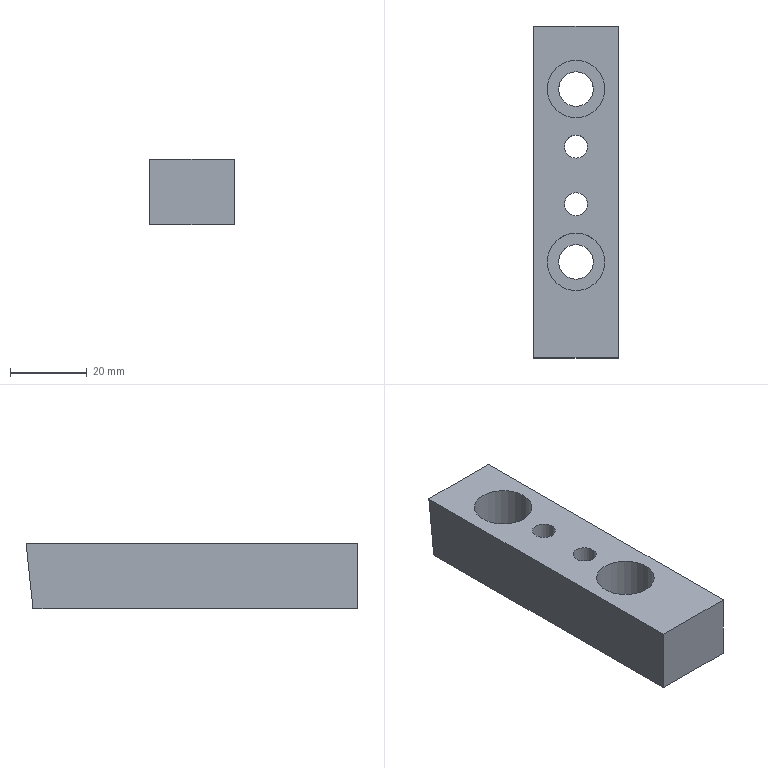Part | NX | features DATUM_CSYS 4, SKETCH 3, CBORE_HOLE 2, HOLE PACKAGE 2, SIMPLE HOLE 2, EXTRUDE 1 | 1 solid | 14 faces | box 22 x 86.4 x 17 mm | volume 26138 mm3 | plane 8 | cylinder 6 | commonest cylinder face diameters 6 x2 9 x2 15 x2
STEP:
#1=CARTESIAN_POINT('',(0.,-43.2,8.5));
#2=VERTEX_POINT('',#1);
#3=CARTESIAN_POINT('',(0.,-43.2,-8.5));
#4=VERTEX_POINT('',#3);
#5=CARTESIAN_POINT('',(0.,-43.2,8.5));
#6=DIRECTION('',(0.,0.,-1.));
#7=VECTOR('',#6,1000.);
#8=LINE('',#5,#7);
#9=EDGE_CURVE('',#2,#4,#8,.T.);
#10=ORIENTED_EDGE('',*,*,#9,.T.);
#11=CARTESIAN_POINT('',(22.,-43.2,-8.5));
#12=VERTEX_POINT('',#11);
#13=CARTESIAN_POINT('',(22.,-43.2,-8.5));
#14=DIRECTION('',(-1.,0.,0.));
#15=VECTOR('',#14,1000.);
#16=LINE('',#13,#15);
#17=EDGE_CURVE('',#12,#4,#16,.T.);
#18=ORIENTED_EDGE('',*,*,#17,.F.);
#19=CARTESIAN_POINT('',(22.,-43.2,8.5));
#20=VERTEX_POINT('',#19);
#21=CARTESIAN_POINT('',(22.,-43.2,8.5));
#22=DIRECTION('',(0.,0.,-1.));
#23=VECTOR('',#22,1000.);
#24=LINE('',#21,#23);
#25=EDGE_CURVE('',#20,#12,#24,.T.);
#26=ORIENTED_EDGE('',*,*,#25,.F.);
#27=CARTESIAN_POINT('',(22.,-43.2,8.5));
#28=DIRECTION('',(-1.,0.,0.));
#29=VECTOR('',#28,1000.);
#30=LINE('',#27,#29);
#31=EDGE_CURVE('',#20,#2,#30,.T.);
#32=ORIENTED_EDGE('',*,*,#31,.T.);
#33=EDGE_LOOP('',(#10,#18,#26,#32));
#34=FACE_BOUND('',#33,.T.);
#35=CARTESIAN_POINT('',(22.,-43.2,8.5));
#36=DIRECTION('',(0.,1.,0.));
#37=DIRECTION('',(0.,0.,1.));
#38=AXIS2_PLACEMENT_3D('',#35,#36,#37);
#39=PLANE('',#38);
#40=ADVANCED_FACE('',(#34),#39,.F.);
#41=CARTESIAN_POINT('',(11.,8.8,-8.5));
#42=VERTEX_POINT('',#41);
#43=CARTESIAN_POINT('',(11.,11.8,-8.5));
#44=DIRECTION('',(0.,0.,1.));
#45=DIRECTION('',(0.,-1.,0.));
#46=AXIS2_PLACEMENT_3D('',#43,#44,#45);
#47=CIRCLE('',#46,3.);
#48=EDGE_CURVE('',#42,#42,#47,.T.);
#49=ORIENTED_EDGE('',*,*,#48,.T.);
#50=EDGE_LOOP('',(#49));
#51=FACE_BOUND('',#50,.T.);
#52=CARTESIAN_POINT('',(11.,-6.2,-8.5));
#53=VERTEX_POINT('',#52);
#54=CARTESIAN_POINT('',(11.,-3.2,-8.5));
#55=DIRECTION('',(0.,0.,1.));
#56=DIRECTION('',(0.,-1.,0.));
#57=AXIS2_PLACEMENT_3D('',#54,#55,#56);
#58=CIRCLE('',#57,3.);
#59=EDGE_CURVE('',#53,#53,#58,.T.);
#60=ORIENTED_EDGE('',*,*,#59,.T.);
#61=EDGE_LOOP('',(#60));
#62=FACE_BOUND('',#61,.T.);
#63=CARTESIAN_POINT('',(11.,22.3,-8.5));
#64=VERTEX_POINT('',#63);
#65=CARTESIAN_POINT('',(11.,26.8,-8.5));
#66=DIRECTION('',(0.,0.,1.));
#67=DIRECTION('',(0.,-1.,0.));
#68=AXIS2_PLACEMENT_3D('',#65,#66,#67);
#69=CIRCLE('',#68,4.5);
#70=EDGE_CURVE('',#64,#64,#69,.T.);
#71=ORIENTED_EDGE('',*,*,#70,.T.);
#72=EDGE_LOOP('',(#71));
#73=FACE_BOUND('',#72,.T.);
#74=CARTESIAN_POINT('',(11.,-22.7,-8.5));
#75=VERTEX_POINT('',#74);
#76=CARTESIAN_POINT('',(11.,-18.2,-8.5));
#77=DIRECTION('',(0.,0.,1.));
#78=DIRECTION('',(0.,-1.,0.));
#79=AXIS2_PLACEMENT_3D('',#76,#77,#78);
#80=CIRCLE('',#79,4.5);
#81=EDGE_CURVE('',#75,#75,#80,.T.);
#82=ORIENTED_EDGE('',*,*,#81,.T.);
#83=EDGE_LOOP('',(#82));
#84=FACE_BOUND('',#83,.T.);
#85=CARTESIAN_POINT('',(0.,41.4,-8.5));
#86=VERTEX_POINT('',#85);
#87=CARTESIAN_POINT('',(0.,-43.2,-8.5));
#88=DIRECTION('',(0.,1.,0.));
#89=VECTOR('',#88,1000.);
#90=LINE('',#87,#89);
#91=EDGE_CURVE('',#4,#86,#90,.T.);
#92=ORIENTED_EDGE('',*,*,#91,.T.);
#93=CARTESIAN_POINT('',(22.,41.4,-8.5));
#94=VERTEX_POINT('',#93);
#95=CARTESIAN_POINT('',(22.,41.4,-8.5));
#96=DIRECTION('',(-1.,0.,0.));
#97=VECTOR('',#96,1000.);
#98=LINE('',#95,#97);
#99=EDGE_CURVE('',#94,#86,#98,.T.);
#100=ORIENTED_EDGE('',*,*,#99,.F.);
#101=CARTESIAN_POINT('',(22.,-43.2,-8.5));
#102=DIRECTION('',(0.,1.,0.));
#103=VECTOR('',#102,1000.);
#104=LINE('',#101,#103);
#105=EDGE_CURVE('',#12,#94,#104,.T.);
#106=ORIENTED_EDGE('',*,*,#105,.F.);
#107=ORIENTED_EDGE('',*,*,#17,.T.);
#108=EDGE_LOOP('',(#92,#100,#106,#107));
#109=FACE_BOUND('',#108,.T.);
#110=CARTESIAN_POINT('',(22.,-43.2,-8.5));
#111=DIRECTION('',(0.,0.,1.));
#112=DIRECTION('',(0.,-1.,0.));
#113=AXIS2_PLACEMENT_3D('',#110,#111,#112);
#114=PLANE('',#113);
#115=ADVANCED_FACE('',(#51,#62,#73,#84,#109),#114,.F.);
#116=CARTESIAN_POINT('',(0.,43.2,8.5));
#117=VERTEX_POINT('',#116);
#118=CARTESIAN_POINT('',(0.,41.4,-8.5));
#119=DIRECTION('',(0.,0.1053,0.9944));
#120=VECTOR('',#119,1000.);
#121=LINE('',#118,#120);
#122=EDGE_CURVE('',#86,#117,#121,.T.);
#123=ORIENTED_EDGE('',*,*,#122,.T.);
#124=CARTESIAN_POINT('',(22.,43.2,8.5));
#125=VERTEX_POINT('',#124);
#126=CARTESIAN_POINT('',(22.,43.2,8.5));
#127=DIRECTION('',(-1.,0.,0.));
#128=VECTOR('',#127,1000.);
#129=LINE('',#126,#128);
#130=EDGE_CURVE('',#125,#117,#129,.T.);
#131=ORIENTED_EDGE('',*,*,#130,.F.);
#132=CARTESIAN_POINT('',(22.,41.4,-8.5));
#133=DIRECTION('',(0.,0.1053,0.9944));
#134=VECTOR('',#133,1000.);
#135=LINE('',#132,#134);
#136=EDGE_CURVE('',#94,#125,#135,.T.);
#137=ORIENTED_EDGE('',*,*,#136,.F.);
#138=ORIENTED_EDGE('',*,*,#99,.T.);
#139=EDGE_LOOP('',(#123,#131,#137,#138));
#140=FACE_BOUND('',#139,.T.);
#141=CARTESIAN_POINT('',(22.,41.4,-8.5));
#142=DIRECTION('',(0.,-0.9944,0.1053));
#143=DIRECTION('',(0.,-0.1053,-0.9944));
#144=AXIS2_PLACEMENT_3D('',#141,#142,#143);
#145=PLANE('',#144);
#146=ADVANCED_FACE('',(#140),#145,.F.);
#147=CARTESIAN_POINT('',(11.,14.8,8.5));
#148=VERTEX_POINT('',#147);
#149=CARTESIAN_POINT('',(11.,11.8,8.5));
#150=DIRECTION('',(0.,0.,-1.));
#151=DIRECTION('',(0.,1.,0.));
#152=AXIS2_PLACEMENT_3D('',#149,#150,#151);
#153=CIRCLE('',#152,3.);
#154=EDGE_CURVE('',#148,#148,#153,.T.);
#155=ORIENTED_EDGE('',*,*,#154,.T.);
#156=EDGE_LOOP('',(#155));
#157=FACE_BOUND('',#156,.T.);
#158=CARTESIAN_POINT('',(11.,-0.2,8.5));
#159=VERTEX_POINT('',#158);
#160=CARTESIAN_POINT('',(11.,-3.2,8.5));
#161=DIRECTION('',(0.,0.,-1.));
#162=DIRECTION('',(0.,1.,0.));
#163=AXIS2_PLACEMENT_3D('',#160,#161,#162);
#164=CIRCLE('',#163,3.);
#165=EDGE_CURVE('',#159,#159,#164,.T.);
#166=ORIENTED_EDGE('',*,*,#165,.T.);
#167=EDGE_LOOP('',(#166));
#168=FACE_BOUND('',#167,.T.);
#169=CARTESIAN_POINT('',(11.,34.3,8.5));
#170=VERTEX_POINT('',#169);
#171=CARTESIAN_POINT('',(11.,26.8,8.5));
#172=DIRECTION('',(0.,0.,-1.));
#173=DIRECTION('',(0.,1.,0.));
#174=AXIS2_PLACEMENT_3D('',#171,#172,#173);
#175=CIRCLE('',#174,7.5);
#176=EDGE_CURVE('',#170,#170,#175,.T.);
#177=ORIENTED_EDGE('',*,*,#176,.T.);
#178=EDGE_LOOP('',(#177));
#179=FACE_BOUND('',#178,.T.);
#180=CARTESIAN_POINT('',(11.,-10.7,8.5));
#181=VERTEX_POINT('',#180);
#182=CARTESIAN_POINT('',(11.,-18.2,8.5));
#183=DIRECTION('',(0.,0.,-1.));
#184=DIRECTION('',(0.,1.,0.));
#185=AXIS2_PLACEMENT_3D('',#182,#183,#184);
#186=CIRCLE('',#185,7.5);
#187=EDGE_CURVE('',#181,#181,#186,.T.);
#188=ORIENTED_EDGE('',*,*,#187,.T.);
#189=EDGE_LOOP('',(#188));
#190=FACE_BOUND('',#189,.T.);
#191=CARTESIAN_POINT('',(0.,43.2,8.5));
#192=DIRECTION('',(0.,-1.,0.));
#193=VECTOR('',#192,1000.);
#194=LINE('',#191,#193);
#195=EDGE_CURVE('',#117,#2,#194,.T.);
#196=ORIENTED_EDGE('',*,*,#195,.T.);
#197=ORIENTED_EDGE('',*,*,#31,.F.);
#198=CARTESIAN_POINT('',(22.,43.2,8.5));
#199=DIRECTION('',(0.,-1.,0.));
#200=VECTOR('',#199,1000.);
#201=LINE('',#198,#200);
#202=EDGE_CURVE('',#125,#20,#201,.T.);
#203=ORIENTED_EDGE('',*,*,#202,.F.);
#204=ORIENTED_EDGE('',*,*,#130,.T.);
#205=EDGE_LOOP('',(#196,#197,#203,#204));
#206=FACE_BOUND('',#205,.T.);
#207=CARTESIAN_POINT('',(22.,43.2,8.5));
#208=DIRECTION('',(0.,0.,-1.));
#209=DIRECTION('',(0.,1.,0.));
#210=AXIS2_PLACEMENT_3D('',#207,#208,#209);
#211=PLANE('',#210);
#212=ADVANCED_FACE('',(#157,#168,#179,#190,#206),#211,.F.);
#213=ORIENTED_EDGE('',*,*,#25,.T.);
#214=ORIENTED_EDGE('',*,*,#105,.T.);
#215=ORIENTED_EDGE('',*,*,#136,.T.);
#216=ORIENTED_EDGE('',*,*,#202,.T.);
#217=EDGE_LOOP('',(#213,#214,#215,#216));
#218=FACE_BOUND('',#217,.T.);
#219=CARTESIAN_POINT('',(22.,0.,0.));
#220=DIRECTION('',(1.,0.,0.));
#221=DIRECTION('',(0.,0.,-1.));
#222=AXIS2_PLACEMENT_3D('',#219,#220,#221);
#223=PLANE('',#222);
#224=ADVANCED_FACE('',(#218),#223,.T.);
#225=ORIENTED_EDGE('',*,*,#9,.F.);
#226=ORIENTED_EDGE('',*,*,#195,.F.);
#227=ORIENTED_EDGE('',*,*,#122,.F.);
#228=ORIENTED_EDGE('',*,*,#91,.F.);
#229=EDGE_LOOP('',(#225,#226,#227,#228));
#230=FACE_BOUND('',#229,.T.);
#231=CARTESIAN_POINT('',(0.,0.,0.));
#232=DIRECTION('',(1.,0.,0.));
#233=DIRECTION('',(0.,0.,-1.));
#234=AXIS2_PLACEMENT_3D('',#231,#232,#233);
#235=PLANE('',#234);
#236=ADVANCED_FACE('',(#230),#235,.F.);
#237=CARTESIAN_POINT('',(11.,-13.7,-3.5));
#238=VERTEX_POINT('',#237);
#239=CARTESIAN_POINT('',(11.,-18.2,-3.5));
#240=DIRECTION('',(0.,0.,-1.));
#241=DIRECTION('',(0.,1.,0.));
#242=AXIS2_PLACEMENT_3D('',#239,#240,#241);
#243=CIRCLE('',#242,4.5);
#244=EDGE_CURVE('',#238,#238,#243,.F.);
#245=ORIENTED_EDGE('',*,*,#244,.T.);
#246=EDGE_LOOP('',(#245));
#247=FACE_BOUND('',#246,.T.);
#248=ORIENTED_EDGE('',*,*,#81,.F.);
#249=EDGE_LOOP('',(#248));
#250=FACE_BOUND('',#249,.T.);
#251=CARTESIAN_POINT('',(11.,-18.2,-41.5));
#252=DIRECTION('',(0.,0.,-1.));
#253=DIRECTION('',(0.,1.,0.));
#254=AXIS2_PLACEMENT_3D('',#251,#252,#253);
#255=CYLINDRICAL_SURFACE('',#254,4.5);
#256=ADVANCED_FACE('',(#247,#250),#255,.F.);
#257=ORIENTED_EDGE('',*,*,#244,.F.);
#258=EDGE_LOOP('',(#257));
#259=FACE_BOUND('',#258,.T.);
#260=CARTESIAN_POINT('',(11.,-10.7,-3.5));
#261=VERTEX_POINT('',#260);
#262=CARTESIAN_POINT('',(11.,-18.2,-3.5));
#263=DIRECTION('',(0.,0.,-1.));
#264=DIRECTION('',(0.,1.,0.));
#265=AXIS2_PLACEMENT_3D('',#262,#263,#264);
#266=CIRCLE('',#265,7.5);
#267=EDGE_CURVE('',#261,#261,#266,.F.);
#268=ORIENTED_EDGE('',*,*,#267,.T.);
#269=EDGE_LOOP('',(#268));
#270=FACE_BOUND('',#269,.T.);
#271=CARTESIAN_POINT('',(11.,-18.2,-3.5));
#272=DIRECTION('',(0.,0.,-1.));
#273=DIRECTION('',(0.,1.,0.));
#274=AXIS2_PLACEMENT_3D('',#271,#272,#273);
#275=PLANE('',#274);
#276=ADVANCED_FACE('',(#259,#270),#275,.F.);
#277=ORIENTED_EDGE('',*,*,#267,.F.);
#278=EDGE_LOOP('',(#277));
#279=FACE_BOUND('',#278,.T.);
#280=ORIENTED_EDGE('',*,*,#187,.F.);
#281=EDGE_LOOP('',(#280));
#282=FACE_BOUND('',#281,.T.);
#283=CARTESIAN_POINT('',(11.,-18.2,8.5));
#284=DIRECTION('',(0.,0.,-1.));
#285=DIRECTION('',(0.,1.,0.));
#286=AXIS2_PLACEMENT_3D('',#283,#284,#285);
#287=CYLINDRICAL_SURFACE('',#286,7.5);
#288=ADVANCED_FACE('',(#279,#282),#287,.F.);
#289=CARTESIAN_POINT('',(11.,31.3,-3.5));
#290=VERTEX_POINT('',#289);
#291=CARTESIAN_POINT('',(11.,26.8,-3.5));
#292=DIRECTION('',(0.,0.,-1.));
#293=DIRECTION('',(0.,1.,0.));
#294=AXIS2_PLACEMENT_3D('',#291,#292,#293);
#295=CIRCLE('',#294,4.5);
#296=EDGE_CURVE('',#290,#290,#295,.F.);
#297=ORIENTED_EDGE('',*,*,#296,.T.);
#298=EDGE_LOOP('',(#297));
#299=FACE_BOUND('',#298,.T.);
#300=ORIENTED_EDGE('',*,*,#70,.F.);
#301=EDGE_LOOP('',(#300));
#302=FACE_BOUND('',#301,.T.);
#303=CARTESIAN_POINT('',(11.,26.8,-41.5));
#304=DIRECTION('',(0.,0.,-1.));
#305=DIRECTION('',(0.,1.,0.));
#306=AXIS2_PLACEMENT_3D('',#303,#304,#305);
#307=CYLINDRICAL_SURFACE('',#306,4.5);
#308=ADVANCED_FACE('',(#299,#302),#307,.F.);
#309=ORIENTED_EDGE('',*,*,#296,.F.);
#310=EDGE_LOOP('',(#309));
#311=FACE_BOUND('',#310,.T.);
#312=CARTESIAN_POINT('',(11.,34.3,-3.5));
#313=VERTEX_POINT('',#312);
#314=CARTESIAN_POINT('',(11.,26.8,-3.5));
#315=DIRECTION('',(0.,0.,-1.));
#316=DIRECTION('',(0.,1.,0.));
#317=AXIS2_PLACEMENT_3D('',#314,#315,#316);
#318=CIRCLE('',#317,7.5);
#319=EDGE_CURVE('',#313,#313,#318,.F.);
#320=ORIENTED_EDGE('',*,*,#319,.T.);
#321=EDGE_LOOP('',(#320));
#322=FACE_BOUND('',#321,.T.);
#323=CARTESIAN_POINT('',(11.,26.8,-3.5));
#324=DIRECTION('',(0.,0.,-1.));
#325=DIRECTION('',(0.,1.,0.));
#326=AXIS2_PLACEMENT_3D('',#323,#324,#325);
#327=PLANE('',#326);
#328=ADVANCED_FACE('',(#311,#322),#327,.F.);
#329=ORIENTED_EDGE('',*,*,#319,.F.);
#330=EDGE_LOOP('',(#329));
#331=FACE_BOUND('',#330,.T.);
#332=ORIENTED_EDGE('',*,*,#176,.F.);
#333=EDGE_LOOP('',(#332));
#334=FACE_BOUND('',#333,.T.);
#335=CARTESIAN_POINT('',(11.,26.8,8.5));
#336=DIRECTION('',(0.,0.,-1.));
#337=DIRECTION('',(0.,1.,0.));
#338=AXIS2_PLACEMENT_3D('',#335,#336,#337);
#339=CYLINDRICAL_SURFACE('',#338,7.5);
#340=ADVANCED_FACE('',(#331,#334),#339,.F.);
#341=ORIENTED_EDGE('',*,*,#165,.F.);
#342=EDGE_LOOP('',(#341));
#343=FACE_BOUND('',#342,.T.);
#344=ORIENTED_EDGE('',*,*,#59,.F.);
#345=EDGE_LOOP('',(#344));
#346=FACE_BOUND('',#345,.T.);
#347=CARTESIAN_POINT('',(11.,-3.2,8.5));
#348=DIRECTION('',(0.,0.,-1.));
#349=DIRECTION('',(0.,1.,0.));
#350=AXIS2_PLACEMENT_3D('',#347,#348,#349);
#351=CYLINDRICAL_SURFACE('',#350,3.);
#352=ADVANCED_FACE('',(#343,#346),#351,.F.);
#353=ORIENTED_EDGE('',*,*,#154,.F.);
#354=EDGE_LOOP('',(#353));
#355=FACE_BOUND('',#354,.T.);
#356=ORIENTED_EDGE('',*,*,#48,.F.);
#357=EDGE_LOOP('',(#356));
#358=FACE_BOUND('',#357,.T.);
#359=CARTESIAN_POINT('',(11.,11.8,8.5));
#360=DIRECTION('',(0.,0.,-1.));
#361=DIRECTION('',(0.,1.,0.));
#362=AXIS2_PLACEMENT_3D('',#359,#360,#361);
#363=CYLINDRICAL_SURFACE('',#362,3.);
#364=ADVANCED_FACE('',(#355,#358),#363,.F.);
#365=CLOSED_SHELL('',(#40,#115,#146,#212,#224,#236,#256,#276,#288,#308,#328,#340,#352,#364));
#366=MANIFOLD_SOLID_BREP('',#365);
#367=(LENGTH_UNIT()NAMED_UNIT(*)SI_UNIT(.MILLI.,.METRE.));
#368=UNCERTAINTY_MEASURE_WITH_UNIT(LENGTH_MEASURE(0.00001),#367,'','');
#369=(NAMED_UNIT(*)PLANE_ANGLE_UNIT()SI_UNIT($,.RADIAN.));
#370=(NAMED_UNIT(*)SI_UNIT($,.STERADIAN.)SOLID_ANGLE_UNIT());
#371=(GEOMETRIC_REPRESENTATION_CONTEXT(3)GLOBAL_UNCERTAINTY_ASSIGNED_CONTEXT((#368))GLOBAL_UNIT_ASSIGNED_CONTEXT((#367,#369,#370))REPRESENTATION_CONTEXT('',''));
#372=ADVANCED_BREP_SHAPE_REPRESENTATION('',(#366),#371);